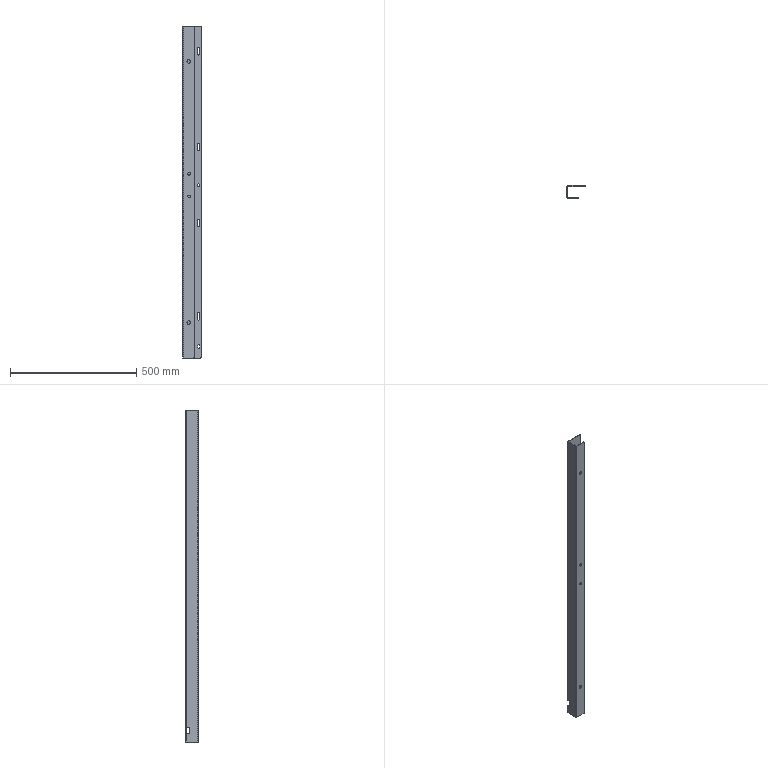Part | 1 solid | 66 faces | box 71.5 x 50 x 1315 mm | volume 620368 mm3 | plane 36 | cylinder 30 | commonest cylinder face diameters 10 x10 4 x4 11 x4 14 x4 0.4 x3 6.4 x3